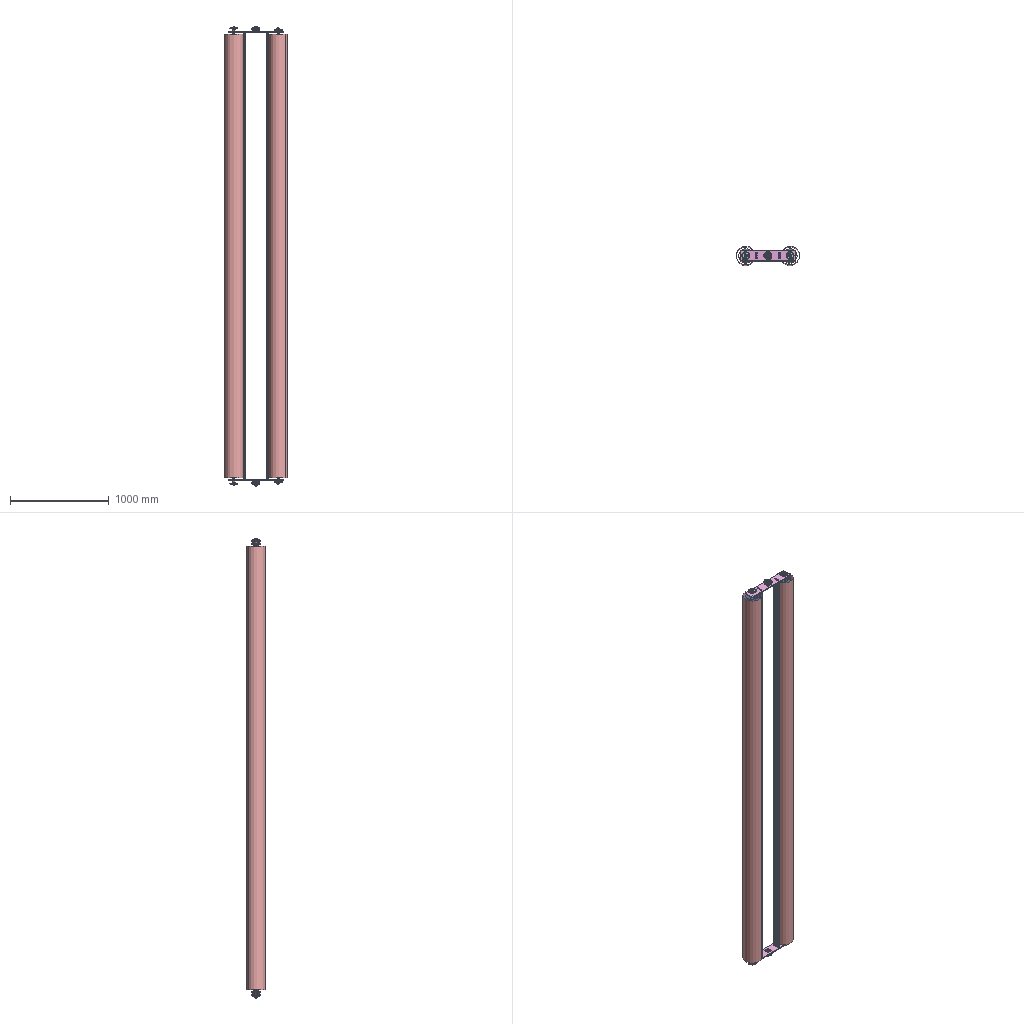Assembly | SolidWorks | 26 different items | 38 placed | box 639 x 190 x 4668 mm
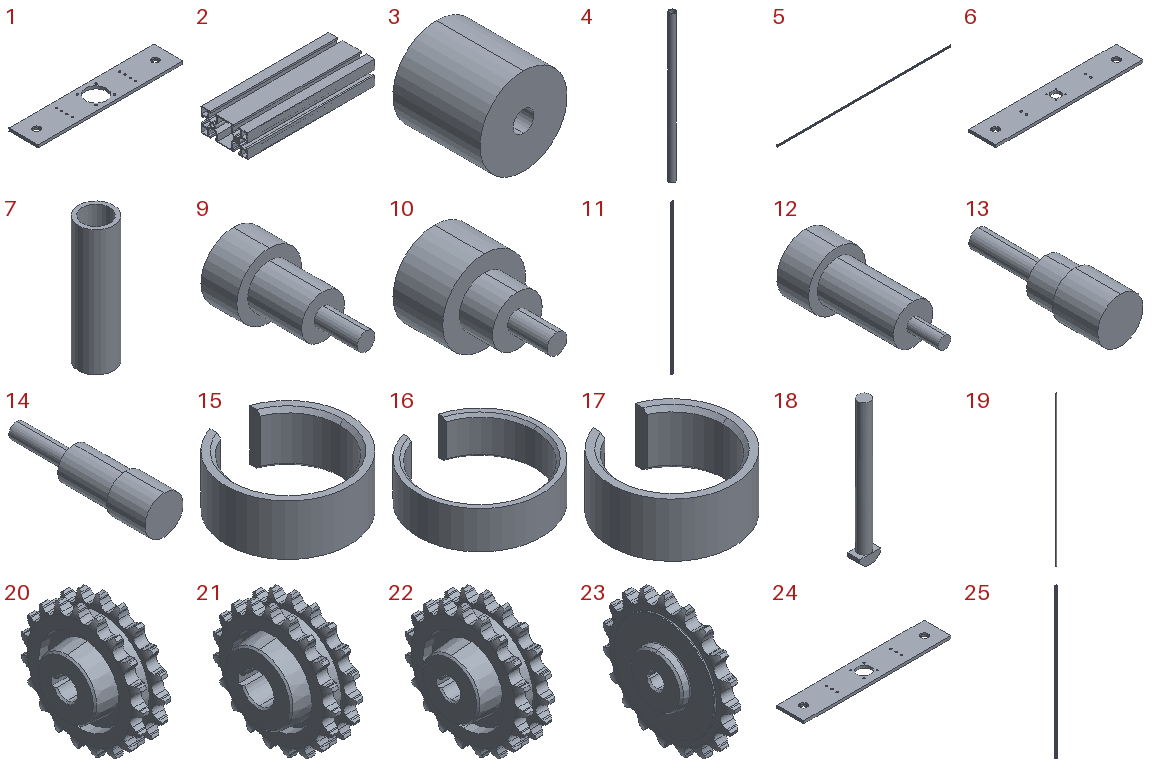Parts list (item | name | quantity | size | volume | features):
1 | - | x1 | 550 x 110 x 10 mm | 540695 mm3 | features ICE 5, Extrusion 1, Fillet 1, HoleWzd 1, MirrorPattern 1
2 | - | x1 | 220 x 80 x 40 mm | 163035 mm3 | features WeldMemberFeat 1, WeldmentFeature 1
3 | - | x1 | 25 x 25 x 25 mm | 11565 mm3 | features Extrusion 1
4 | - | x2 | 190 x 190 x 4500 mm | 116967 mm3 | features Extrusion 1, ICE 1
5 | - | x1 | 4546 x 20 x 40 mm | 1364953 mm3 | features HoleWzd 1, WeldMemberFeat 1, WeldmentFeature 1
6 | - | x1 | 550 x 100 x 10 mm | 528570 mm3 | features ICE 5, Extrusion 1, Fillet 1, HoleWzd 1, MirrorPattern 1
7 | - | x1 | 9 x 9 x 32 mm | 804.248 mm3 | features Extrusion 1
8 | - | x1 | - | - | features Boss 3, CurvePattern 2, Chamfer 1, CompositeCurve 1, Extrusion 1, MirrorPattern 1, MirrorSolid 1
9 | - | x2 | 18 x 37 x 18 mm | 4200 mm3 | features ICE 3, Extrusion 1
10 | - | x1 | 25 x 37 x 25 mm | 7911 mm3 | features ICE 3, Extrusion 1
11 | - | x1 | 80 x 20 x 4546 mm | 2507089 mm3 | features MBimport 1, MoveFace 1
12 | - | x1 | 18 x 44 x 18 mm | 5338 mm3 | features ICE 3, Extrusion 1
13 | - | x2 | 20 x 62.8 x 20 mm | 10660 mm3 | features ICE 3, Extrusion 1
14 | - | x2 | 20 x 77.2 x 20 mm | 13929 mm3 | features ICE 3, Extrusion 1
15 | - | x2 | 17 x 16.543 x 7 mm | 415.187 mm3 | features Chamfer 1, Extrusion 1, ICE 1
16 | - | x1 | 23 x 22.531 x 7 mm | 585.831 mm3 | features Chamfer 1, Extrusion 1, ICE 1
17 | - | x1 | 16 x 15.512 x 7 mm | 385.007 mm3 | features Chamfer 1, Extrusion 1, ICE 1
18 | - | x1 | 10 x 6 x 69.5 mm | 2064 mm3 | features Extrusion 1, ICE 1
19 | - | x2 | 35 x 35 x 4500 mm | 1357168 mm3 | features Extrusion 1
20 | - | x2 | 40 x 81.595 x 81.862 mm | 93771 mm3 | features Cut 2, Revolution 2, Chamfer 1, CirPattern 1, LPattern 1
21 | - | x1 | 40 x 81.595 x 81.862 mm | 99191 mm3 | features Cut 2, Revolution 2, Chamfer 1, CirPattern 1, LPattern 1
22 | - | x1 | 40 x 81.595 x 81.862 mm | 92773 mm3 | features Cut 2, Revolution 2, Chamfer 1, CirPattern 1, LPattern 1
23 | - | x4 | 20 x 81.595 x 81.862 mm | 45176 mm3 | features Cut 2, Revolution 2, Chamfer 1, CirPattern 1, Fillet 1, MirrorPattern 1
24 | - | x2 | 550 x 100 x 10 mm | 517578 mm3 | features ICE 5, Extrusion 1, Fillet 1, HoleWzd 1, MirrorPattern 1
25 | - | x2 | 60 x 20 x 4546 mm | 1925976 mm3 | features MBimport 1, MoveFace 1
26 | deep groove ball bearings gb | x1 | - | - | -
Mates (type | each side: item.copy, entity, surface, feature):
Coincident | 25.1 face plane 2060 profile.step | 24.1 face plane Boss-Extrude1
Coincident | 25.2 face plane 2060 profile.step | 24.1 face plane Boss-Extrude1
Concentric | 25.1 face cylinder 2060 profile.step | 24.1 face cylinder Cut-Extrude6 | 2 times
Concentric | 25.2 face cylinder 2060 profile.step | 24.1 face cylinder Cut-Extrude6 | 2 times
Coincident | 25.1 face plane 2060 profile.step | 24.2 face plane Boss-Extrude1
Concentric | 25.1 face cylinder 2060 profile.step | 24.2 face cylinder Cut-Extrude6 | 2 times
Concentric | 25.2 face cylinder 2060 profile.step | 24.2 face cylinder Cut-Extrude6 | 2 times
Coincident | 24.1 face plane Boss-Extrude1 | 13.1 face plane Boss-Extrude1
Coincident | 20.1 face plane Revolve2 | 15.1 face plane Boss-Extrude1
Concentric | 20.1 face cylinder Revolve2 | 9.1 face cylinder Boss-Extrude2
Coincident | 20.1 face plane Revolve2 | 9.1 face plane Boss-Extrude3
Coincident | 15.2 face plane Boss-Extrude1 | 20.2 face plane Revolve2
Concentric | 20.2 face cylinder Revolve2 | 9.2 face cylinder Boss-Extrude2
Coincident | 20.2 face plane Revolve2 | 9.2 face plane Boss-Extrude3
Coincident | 24.2 face plane Boss-Extrude1 | 14.1 face plane Boss-Extrude1
Coincident | 24.1 face plane Boss-Extrude1 | 14.2 face plane Boss-Extrude1
Concentric | 13.1 face cylinder Boss-Extrude3 | 23.1 face cylinder Revolve1
Coincident | 13.1 face plane Boss-Extrude2 | 23.1 face plane Revolve2
Concentric | 14.2 face cylinder Boss-Extrude3 | 23.2 face cylinder Revolve1
Coincident | 14.2 face plane Boss-Extrude2 | 23.2 face plane Revolve2
Concentric | 13.2 face cylinder Boss-Extrude3 | 23.3 face cylinder Revolve1
Coincident | 13.2 face plane Boss-Extrude2 | 23.3 face plane Revolve2
Concentric | 14.1 face cylinder Boss-Extrude3 | 23.4 face cylinder Revolve1
Coincident | 14.1 face plane Boss-Extrude2 | 23.4 face plane Revolve2
Coincident | 14.1 face plane Cut-Extrude1 | 23.4 face plane Cut-Extrude2
Coincident | 13.2 face plane Cut-Extrude1 | 23.3 face plane Cut-Extrude2
Coincident | 14.2 face plane Cut-Extrude1 | 23.2 face plane Cut-Extrude2
Coincident | 13.1 face plane Cut-Extrude1 | 23.1 face plane Cut-Extrude2
Concentric | 4.1 face cylinder Boss-Extrude2 | 19.1 face cylinder Boss-Extrude1
Concentric | 4.2 face cylinder Boss-Extrude2 | 19.2 face cylinder Boss-Extrude1